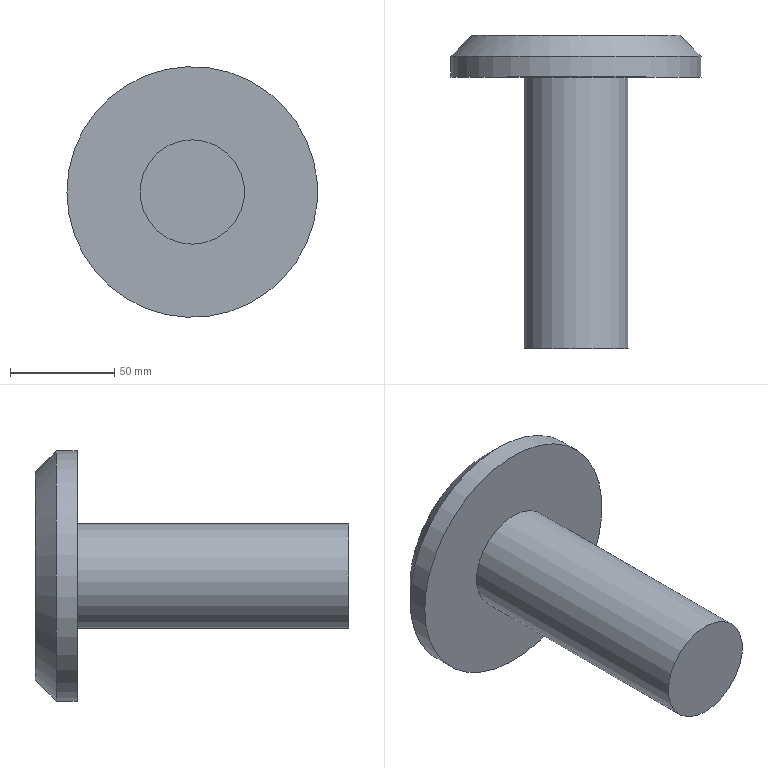Part | NX | features solid 2 | 1 solid | 6 faces | box 120 x 150 x 120 mm | volume 463647 mm3 | plane 3 | cylinder 2 | cone 1 | commonest cylinder face diameters 50 x1 120 x1
STEP:
#1=CARTESIAN_POINT('',(605.,440.,-190.));
#2=VERTEX_POINT('',#1);
#3=CARTESIAN_POINT('',(605.,440.,-165.));
#4=DIRECTION('',(0.,-1.,0.));
#5=DIRECTION('',(0.,0.,-1.));
#6=AXIS2_PLACEMENT_3D('',#3,#4,#5);
#7=CIRCLE('',#6,25.);
#8=EDGE_CURVE('',#2,#2,#7,.F.);
#9=ORIENTED_EDGE('',*,*,#8,.F.);
#10=EDGE_LOOP('',(#9));
#11=FACE_BOUND('',#10,.T.);
#12=CARTESIAN_POINT('',(605.,310.,-140.));
#13=VERTEX_POINT('',#12);
#14=CARTESIAN_POINT('',(605.,310.,-165.));
#15=DIRECTION('',(0.,1.,0.));
#16=DIRECTION('',(0.,0.,1.));
#17=AXIS2_PLACEMENT_3D('',#14,#15,#16);
#18=CIRCLE('',#17,25.);
#19=EDGE_CURVE('',#13,#13,#18,.F.);
#20=ORIENTED_EDGE('',*,*,#19,.F.);
#21=EDGE_LOOP('',(#20));
#22=FACE_BOUND('',#21,.T.);
#23=CARTESIAN_POINT('',(605.,440.,-165.));
#24=DIRECTION('',(0.,-1.,0.));
#25=DIRECTION('',(0.,0.,-1.));
#26=AXIS2_PLACEMENT_3D('',#23,#24,#25);
#27=CYLINDRICAL_SURFACE('',#26,25.);
#28=ADVANCED_FACE('',(#11,#22),#27,.T.);
#29=ORIENTED_EDGE('',*,*,#19,.T.);
#30=EDGE_LOOP('',(#29));
#31=FACE_BOUND('',#30,.T.);
#32=CARTESIAN_POINT('',(605.,310.,-165.));
#33=DIRECTION('',(0.,-1.,0.));
#34=DIRECTION('',(0.,0.,-1.));
#35=AXIS2_PLACEMENT_3D('',#32,#33,#34);
#36=PLANE('',#35);
#37=ADVANCED_FACE('',(#31),#36,.T.);
#38=CARTESIAN_POINT('',(545.,450.,-165.));
#39=VERTEX_POINT('',#38);
#40=CARTESIAN_POINT('',(605.,450.,-165.));
#41=DIRECTION('',(0.,-1.,0.));
#42=DIRECTION('',(-1.,0.,0.));
#43=AXIS2_PLACEMENT_3D('',#40,#41,#42);
#44=CIRCLE('',#43,60.);
#45=EDGE_CURVE('',#39,#39,#44,.T.);
#46=ORIENTED_EDGE('',*,*,#45,.T.);
#47=EDGE_LOOP('',(#46));
#48=FACE_BOUND('',#47,.T.);
#49=CARTESIAN_POINT('',(545.,440.,-165.));
#50=VERTEX_POINT('',#49);
#51=CARTESIAN_POINT('',(605.,440.,-165.));
#52=DIRECTION('',(0.,-1.,0.));
#53=DIRECTION('',(-1.,0.,0.));
#54=AXIS2_PLACEMENT_3D('',#51,#52,#53);
#55=CIRCLE('',#54,60.);
#56=EDGE_CURVE('',#50,#50,#55,.T.);
#57=ORIENTED_EDGE('',*,*,#56,.F.);
#58=EDGE_LOOP('',(#57));
#59=FACE_BOUND('',#58,.T.);
#60=CARTESIAN_POINT('',(605.,450.,-165.));
#61=DIRECTION('',(0.,-1.,0.));
#62=DIRECTION('',(0.,0.,-1.));
#63=AXIS2_PLACEMENT_3D('',#60,#61,#62);
#64=CYLINDRICAL_SURFACE('',#63,60.);
#65=ADVANCED_FACE('',(#48,#59),#64,.T.);
#66=ORIENTED_EDGE('',*,*,#8,.T.);
#67=EDGE_LOOP('',(#66));
#68=FACE_BOUND('',#67,.T.);
#69=ORIENTED_EDGE('',*,*,#56,.T.);
#70=EDGE_LOOP('',(#69));
#71=FACE_BOUND('',#70,.T.);
#72=CARTESIAN_POINT('',(605.,440.,-165.));
#73=DIRECTION('',(0.,-1.,0.));
#74=DIRECTION('',(0.,0.,-1.));
#75=AXIS2_PLACEMENT_3D('',#72,#73,#74);
#76=PLANE('',#75);
#77=ADVANCED_FACE('',(#68,#71),#76,.T.);
#78=CARTESIAN_POINT('',(605.,460.,-215.));
#79=VERTEX_POINT('',#78);
#80=CARTESIAN_POINT('',(605.,460.,-165.));
#81=DIRECTION('',(0.,-1.,0.));
#82=DIRECTION('',(0.,0.,-1.));
#83=AXIS2_PLACEMENT_3D('',#80,#81,#82);
#84=CIRCLE('',#83,50.);
#85=EDGE_CURVE('',#79,#79,#84,.T.);
#86=ORIENTED_EDGE('',*,*,#85,.T.);
#87=EDGE_LOOP('',(#86));
#88=FACE_BOUND('',#87,.T.);
#89=ORIENTED_EDGE('',*,*,#45,.F.);
#90=EDGE_LOOP('',(#89));
#91=FACE_BOUND('',#90,.T.);
#92=CARTESIAN_POINT('',(605.,450.,-165.));
#93=DIRECTION('',(0.,-1.,0.));
#94=DIRECTION('',(0.,0.,1.));
#95=AXIS2_PLACEMENT_3D('',#92,#93,#94);
#96=CONICAL_SURFACE('',#95,60.,0.7854);
#97=ADVANCED_FACE('',(#88,#91),#96,.T.);
#98=ORIENTED_EDGE('',*,*,#85,.F.);
#99=EDGE_LOOP('',(#98));
#100=FACE_BOUND('',#99,.T.);
#101=CARTESIAN_POINT('',(605.,460.,-165.));
#102=DIRECTION('',(0.,-1.,0.));
#103=DIRECTION('',(0.,0.,-1.));
#104=AXIS2_PLACEMENT_3D('',#101,#102,#103);
#105=PLANE('',#104);
#106=ADVANCED_FACE('',(#100),#105,.F.);
#107=CLOSED_SHELL('',(#28,#37,#65,#77,#97,#106));
#108=MANIFOLD_SOLID_BREP('',#107);
#109=(LENGTH_UNIT()NAMED_UNIT(*)SI_UNIT(.MILLI.,.METRE.));
#110=UNCERTAINTY_MEASURE_WITH_UNIT(LENGTH_MEASURE(0.00001),#109,'','');
#111=(NAMED_UNIT(*)PLANE_ANGLE_UNIT()SI_UNIT($,.RADIAN.));
#112=(NAMED_UNIT(*)SI_UNIT($,.STERADIAN.)SOLID_ANGLE_UNIT());
#113=(GEOMETRIC_REPRESENTATION_CONTEXT(3)GLOBAL_UNCERTAINTY_ASSIGNED_CONTEXT((#110))GLOBAL_UNIT_ASSIGNED_CONTEXT((#109,#111,#112))REPRESENTATION_CONTEXT('',''));
#114=ADVANCED_BREP_SHAPE_REPRESENTATION('',(#108),#113);